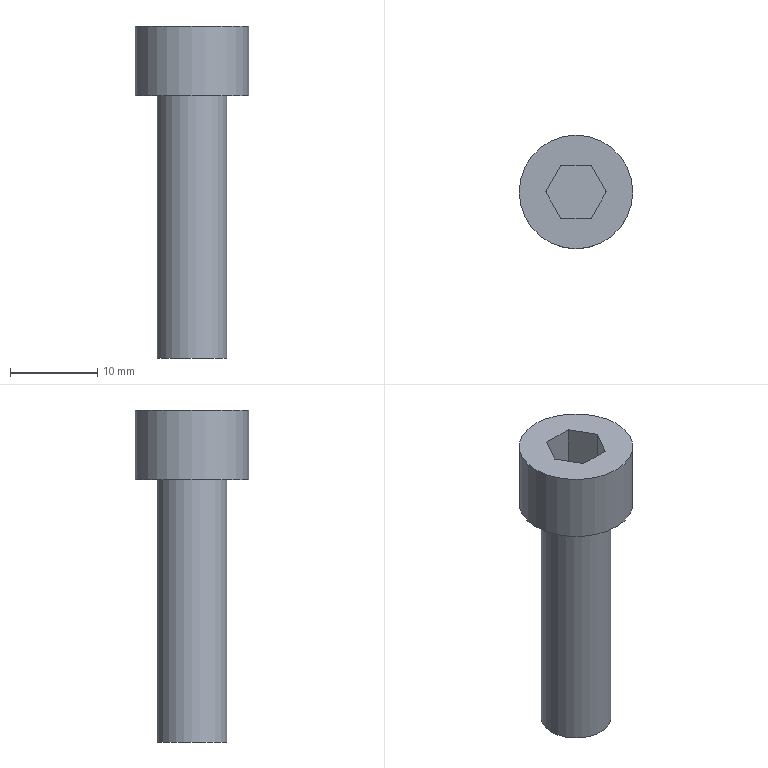Part | STEP file | 冲床-300配套压波_id90_x_t | 1 solid | 12 faces | box 13 x 13 x 38 mm | volume 2405 mm3 | plane 10 | cylinder 2 | commonest cylinder face diameters 8 x1 13 x1
STEP:
#1=CARTESIAN_POINT('',(1171.5,-205.,30.));
#2=VERTEX_POINT('',#1);
#3=CARTESIAN_POINT('',(1165.,-205.,30.));
#4=DIRECTION('',(0.,0.,1.));
#5=DIRECTION('',(1.,0.,0.));
#6=AXIS2_PLACEMENT_3D('',#3,#4,#5);
#7=CIRCLE('',#6,6.5);
#8=EDGE_CURVE('',#2,#2,#7,.T.);
#9=ORIENTED_EDGE('',*,*,#8,.T.);
#10=EDGE_LOOP('',(#9));
#11=FACE_BOUND('',#10,.T.);
#12=CARTESIAN_POINT('',(1166.732,-208.,30.));
#13=VERTEX_POINT('',#12);
#14=CARTESIAN_POINT('',(1163.268,-208.,30.));
#15=VERTEX_POINT('',#14);
#16=CARTESIAN_POINT('',(1163.268,-208.,30.));
#17=DIRECTION('',(-1.,0.,0.));
#18=VECTOR('',#17,1.);
#19=LINE('',#16,#18);
#20=EDGE_CURVE('',#13,#15,#19,.T.);
#21=ORIENTED_EDGE('',*,*,#20,.T.);
#22=CARTESIAN_POINT('',(1161.536,-205.,30.));
#23=VERTEX_POINT('',#22);
#24=CARTESIAN_POINT('',(1161.536,-205.,30.));
#25=DIRECTION('',(-0.5,0.866,0.));
#26=VECTOR('',#25,1.);
#27=LINE('',#24,#26);
#28=EDGE_CURVE('',#15,#23,#27,.T.);
#29=ORIENTED_EDGE('',*,*,#28,.T.);
#30=CARTESIAN_POINT('',(1163.268,-202.,30.));
#31=VERTEX_POINT('',#30);
#32=CARTESIAN_POINT('',(1163.268,-202.,30.));
#33=DIRECTION('',(0.5,0.866,0.));
#34=VECTOR('',#33,1.);
#35=LINE('',#32,#34);
#36=EDGE_CURVE('',#23,#31,#35,.T.);
#37=ORIENTED_EDGE('',*,*,#36,.T.);
#38=CARTESIAN_POINT('',(1166.732,-202.,30.));
#39=VERTEX_POINT('',#38);
#40=CARTESIAN_POINT('',(1166.732,-202.,30.));
#41=DIRECTION('',(1.,0.,0.));
#42=VECTOR('',#41,1.);
#43=LINE('',#40,#42);
#44=EDGE_CURVE('',#31,#39,#43,.T.);
#45=ORIENTED_EDGE('',*,*,#44,.T.);
#46=CARTESIAN_POINT('',(1168.464,-205.,30.));
#47=VERTEX_POINT('',#46);
#48=CARTESIAN_POINT('',(1168.464,-205.,30.));
#49=DIRECTION('',(0.5,-0.866,0.));
#50=VECTOR('',#49,1.);
#51=LINE('',#48,#50);
#52=EDGE_CURVE('',#39,#47,#51,.T.);
#53=ORIENTED_EDGE('',*,*,#52,.T.);
#54=CARTESIAN_POINT('',(1166.732,-208.,30.));
#55=DIRECTION('',(-0.5,-0.866,0.));
#56=VECTOR('',#55,1.);
#57=LINE('',#54,#56);
#58=EDGE_CURVE('',#47,#13,#57,.T.);
#59=ORIENTED_EDGE('',*,*,#58,.T.);
#60=EDGE_LOOP('',(#21,#29,#37,#45,#53,#59));
#61=FACE_BOUND('',#60,.T.);
#62=CARTESIAN_POINT('',(1171.5,-205.,30.));
#63=DIRECTION('',(0.,0.,-1.));
#64=DIRECTION('',(-1.,0.,0.));
#65=AXIS2_PLACEMENT_3D('',#62,#63,#64);
#66=PLANE('',#65);
#67=ADVANCED_FACE('',(#11,#61),#66,.F.);
#68=ORIENTED_EDGE('',*,*,#8,.F.);
#69=EDGE_LOOP('',(#68));
#70=FACE_BOUND('',#69,.T.);
#71=CARTESIAN_POINT('',(1171.5,-205.,22.));
#72=VERTEX_POINT('',#71);
#73=CARTESIAN_POINT('',(1165.,-205.,22.));
#74=DIRECTION('',(0.,0.,1.));
#75=DIRECTION('',(1.,0.,0.));
#76=AXIS2_PLACEMENT_3D('',#73,#74,#75);
#77=CIRCLE('',#76,6.5);
#78=EDGE_CURVE('',#72,#72,#77,.T.);
#79=ORIENTED_EDGE('',*,*,#78,.T.);
#80=EDGE_LOOP('',(#79));
#81=FACE_BOUND('',#80,.T.);
#82=CARTESIAN_POINT('',(1165.,-205.,23.1));
#83=DIRECTION('',(0.,0.,1.));
#84=DIRECTION('',(1.,0.,0.));
#85=AXIS2_PLACEMENT_3D('',#82,#83,#84);
#86=CYLINDRICAL_SURFACE('',#85,6.5);
#87=ADVANCED_FACE('',(#70,#81),#86,.T.);
#88=ORIENTED_EDGE('',*,*,#78,.F.);
#89=EDGE_LOOP('',(#88));
#90=FACE_BOUND('',#89,.T.);
#91=CARTESIAN_POINT('',(1169.,-205.,22.));
#92=VERTEX_POINT('',#91);
#93=CARTESIAN_POINT('',(1165.,-205.,22.));
#94=DIRECTION('',(0.,0.,1.));
#95=DIRECTION('',(1.,0.,0.));
#96=AXIS2_PLACEMENT_3D('',#93,#94,#95);
#97=CIRCLE('',#96,4.);
#98=EDGE_CURVE('',#92,#92,#97,.T.);
#99=ORIENTED_EDGE('',*,*,#98,.T.);
#100=EDGE_LOOP('',(#99));
#101=FACE_BOUND('',#100,.T.);
#102=CARTESIAN_POINT('',(1169.,-205.,22.));
#103=DIRECTION('',(0.,0.,1.));
#104=DIRECTION('',(1.,0.,0.));
#105=AXIS2_PLACEMENT_3D('',#102,#103,#104);
#106=PLANE('',#105);
#107=ADVANCED_FACE('',(#90,#101),#106,.F.);
#108=ORIENTED_EDGE('',*,*,#98,.F.);
#109=EDGE_LOOP('',(#108));
#110=FACE_BOUND('',#109,.T.);
#111=CARTESIAN_POINT('',(1169.,-205.,-8.));
#112=VERTEX_POINT('',#111);
#113=CARTESIAN_POINT('',(1165.,-205.,-8.));
#114=DIRECTION('',(0.,0.,1.));
#115=DIRECTION('',(1.,0.,0.));
#116=AXIS2_PLACEMENT_3D('',#113,#114,#115);
#117=CIRCLE('',#116,4.);
#118=EDGE_CURVE('',#112,#112,#117,.T.);
#119=ORIENTED_EDGE('',*,*,#118,.T.);
#120=EDGE_LOOP('',(#119));
#121=FACE_BOUND('',#120,.T.);
#122=CARTESIAN_POINT('',(1165.,-205.,23.1));
#123=DIRECTION('',(0.,0.,1.));
#124=DIRECTION('',(1.,0.,0.));
#125=AXIS2_PLACEMENT_3D('',#122,#123,#124);
#126=CYLINDRICAL_SURFACE('',#125,4.);
#127=ADVANCED_FACE('',(#110,#121),#126,.T.);
#128=ORIENTED_EDGE('',*,*,#118,.F.);
#129=EDGE_LOOP('',(#128));
#130=FACE_OUTER_BOUND('',#129,.T.);
#131=CARTESIAN_POINT('',(1165.,-205.,-8.));
#132=DIRECTION('',(0.,0.,1.));
#133=DIRECTION('',(1.,0.,0.));
#134=AXIS2_PLACEMENT_3D('',#131,#132,#133);
#135=PLANE('',#134);
#136=ADVANCED_FACE('',(#130),#135,.F.);
#137=ORIENTED_EDGE('',*,*,#20,.F.);
#138=CARTESIAN_POINT('',(1166.732,-208.,24.72));
#139=VERTEX_POINT('',#138);
#140=CARTESIAN_POINT('',(1166.732,-208.,24.72));
#141=DIRECTION('',(0.,0.,1.));
#142=VECTOR('',#141,1.);
#143=LINE('',#140,#142);
#144=EDGE_CURVE('',#139,#13,#143,.T.);
#145=ORIENTED_EDGE('',*,*,#144,.F.);
#146=CARTESIAN_POINT('',(1163.268,-208.,24.72));
#147=VERTEX_POINT('',#146);
#148=CARTESIAN_POINT('',(1163.268,-208.,24.72));
#149=DIRECTION('',(1.,0.,0.));
#150=VECTOR('',#149,1.);
#151=LINE('',#148,#150);
#152=EDGE_CURVE('',#147,#139,#151,.T.);
#153=ORIENTED_EDGE('',*,*,#152,.F.);
#154=CARTESIAN_POINT('',(1163.268,-208.,24.72));
#155=DIRECTION('',(0.,0.,1.));
#156=VECTOR('',#155,1.);
#157=LINE('',#154,#156);
#158=EDGE_CURVE('',#147,#15,#157,.T.);
#159=ORIENTED_EDGE('',*,*,#158,.T.);
#160=EDGE_LOOP('',(#137,#145,#153,#159));
#161=FACE_OUTER_BOUND('',#160,.T.);
#162=CARTESIAN_POINT('',(1163.268,-208.,24.72));
#163=DIRECTION('',(0.,1.,0.));
#164=DIRECTION('',(1.,0.,0.));
#165=AXIS2_PLACEMENT_3D('',#162,#163,#164);
#166=PLANE('',#165);
#167=ADVANCED_FACE('',(#161),#166,.T.);
#168=ORIENTED_EDGE('',*,*,#58,.F.);
#169=CARTESIAN_POINT('',(1168.464,-205.,24.72));
#170=VERTEX_POINT('',#169);
#171=CARTESIAN_POINT('',(1168.464,-205.,24.72));
#172=DIRECTION('',(0.,0.,1.));
#173=VECTOR('',#172,1.);
#174=LINE('',#171,#173);
#175=EDGE_CURVE('',#170,#47,#174,.T.);
#176=ORIENTED_EDGE('',*,*,#175,.F.);
#177=CARTESIAN_POINT('',(1166.732,-208.,24.72));
#178=DIRECTION('',(0.5,0.866,0.));
#179=VECTOR('',#178,1.);
#180=LINE('',#177,#179);
#181=EDGE_CURVE('',#139,#170,#180,.T.);
#182=ORIENTED_EDGE('',*,*,#181,.F.);
#183=ORIENTED_EDGE('',*,*,#144,.T.);
#184=EDGE_LOOP('',(#168,#176,#182,#183));
#185=FACE_OUTER_BOUND('',#184,.T.);
#186=CARTESIAN_POINT('',(1166.732,-208.,24.72));
#187=DIRECTION('',(-0.866,0.5,0.));
#188=DIRECTION('',(0.5,0.866,0.));
#189=AXIS2_PLACEMENT_3D('',#186,#187,#188);
#190=PLANE('',#189);
#191=ADVANCED_FACE('',(#185),#190,.T.);
#192=ORIENTED_EDGE('',*,*,#52,.F.);
#193=CARTESIAN_POINT('',(1166.732,-202.,24.72));
#194=VERTEX_POINT('',#193);
#195=CARTESIAN_POINT('',(1166.732,-202.,24.72));
#196=DIRECTION('',(0.,0.,1.));
#197=VECTOR('',#196,1.);
#198=LINE('',#195,#197);
#199=EDGE_CURVE('',#194,#39,#198,.T.);
#200=ORIENTED_EDGE('',*,*,#199,.F.);
#201=CARTESIAN_POINT('',(1168.464,-205.,24.72));
#202=DIRECTION('',(-0.5,0.866,0.));
#203=VECTOR('',#202,1.);
#204=LINE('',#201,#203);
#205=EDGE_CURVE('',#170,#194,#204,.T.);
#206=ORIENTED_EDGE('',*,*,#205,.F.);
#207=ORIENTED_EDGE('',*,*,#175,.T.);
#208=EDGE_LOOP('',(#192,#200,#206,#207));
#209=FACE_OUTER_BOUND('',#208,.T.);
#210=CARTESIAN_POINT('',(1168.464,-205.,24.72));
#211=DIRECTION('',(-0.866,-0.5,0.));
#212=DIRECTION('',(-0.5,0.866,0.));
#213=AXIS2_PLACEMENT_3D('',#210,#211,#212);
#214=PLANE('',#213);
#215=ADVANCED_FACE('',(#209),#214,.T.);
#216=ORIENTED_EDGE('',*,*,#44,.F.);
#217=CARTESIAN_POINT('',(1163.268,-202.,24.72));
#218=VERTEX_POINT('',#217);
#219=CARTESIAN_POINT('',(1163.268,-202.,24.72));
#220=DIRECTION('',(0.,0.,1.));
#221=VECTOR('',#220,1.);
#222=LINE('',#219,#221);
#223=EDGE_CURVE('',#218,#31,#222,.T.);
#224=ORIENTED_EDGE('',*,*,#223,.F.);
#225=CARTESIAN_POINT('',(1166.732,-202.,24.72));
#226=DIRECTION('',(-1.,0.,0.));
#227=VECTOR('',#226,1.);
#228=LINE('',#225,#227);
#229=EDGE_CURVE('',#194,#218,#228,.T.);
#230=ORIENTED_EDGE('',*,*,#229,.F.);
#231=ORIENTED_EDGE('',*,*,#199,.T.);
#232=EDGE_LOOP('',(#216,#224,#230,#231));
#233=FACE_OUTER_BOUND('',#232,.T.);
#234=CARTESIAN_POINT('',(1166.732,-202.,24.72));
#235=DIRECTION('',(0.,-1.,0.));
#236=DIRECTION('',(-1.,0.,0.));
#237=AXIS2_PLACEMENT_3D('',#234,#235,#236);
#238=PLANE('',#237);
#239=ADVANCED_FACE('',(#233),#238,.T.);
#240=ORIENTED_EDGE('',*,*,#36,.F.);
#241=CARTESIAN_POINT('',(1161.536,-205.,24.72));
#242=VERTEX_POINT('',#241);
#243=CARTESIAN_POINT('',(1161.536,-205.,24.72));
#244=DIRECTION('',(0.,0.,1.));
#245=VECTOR('',#244,1.);
#246=LINE('',#243,#245);
#247=EDGE_CURVE('',#242,#23,#246,.T.);
#248=ORIENTED_EDGE('',*,*,#247,.F.);
#249=CARTESIAN_POINT('',(1163.268,-202.,24.72));
#250=DIRECTION('',(-0.5,-0.866,0.));
#251=VECTOR('',#250,1.);
#252=LINE('',#249,#251);
#253=EDGE_CURVE('',#218,#242,#252,.T.);
#254=ORIENTED_EDGE('',*,*,#253,.F.);
#255=ORIENTED_EDGE('',*,*,#223,.T.);
#256=EDGE_LOOP('',(#240,#248,#254,#255));
#257=FACE_OUTER_BOUND('',#256,.T.);
#258=CARTESIAN_POINT('',(1163.268,-202.,24.72));
#259=DIRECTION('',(0.866,-0.5,0.));
#260=DIRECTION('',(-0.5,-0.866,0.));
#261=AXIS2_PLACEMENT_3D('',#258,#259,#260);
#262=PLANE('',#261);
#263=ADVANCED_FACE('',(#257),#262,.T.);
#264=ORIENTED_EDGE('',*,*,#28,.F.);
#265=ORIENTED_EDGE('',*,*,#158,.F.);
#266=CARTESIAN_POINT('',(1161.536,-205.,24.72));
#267=DIRECTION('',(0.5,-0.866,0.));
#268=VECTOR('',#267,1.);
#269=LINE('',#266,#268);
#270=EDGE_CURVE('',#242,#147,#269,.T.);
#271=ORIENTED_EDGE('',*,*,#270,.F.);
#272=ORIENTED_EDGE('',*,*,#247,.T.);
#273=EDGE_LOOP('',(#264,#265,#271,#272));
#274=FACE_OUTER_BOUND('',#273,.T.);
#275=CARTESIAN_POINT('',(1161.536,-205.,24.72));
#276=DIRECTION('',(0.866,0.5,0.));
#277=DIRECTION('',(0.5,-0.866,0.));
#278=AXIS2_PLACEMENT_3D('',#275,#276,#277);
#279=PLANE('',#278);
#280=ADVANCED_FACE('',(#274),#279,.T.);
#281=ORIENTED_EDGE('',*,*,#152,.T.);
#282=ORIENTED_EDGE('',*,*,#181,.T.);
#283=ORIENTED_EDGE('',*,*,#205,.T.);
#284=ORIENTED_EDGE('',*,*,#229,.T.);
#285=ORIENTED_EDGE('',*,*,#253,.T.);
#286=ORIENTED_EDGE('',*,*,#270,.T.);
#287=EDGE_LOOP('',(#281,#282,#283,#284,#285,#286));
#288=FACE_OUTER_BOUND('',#287,.T.);
#289=CARTESIAN_POINT('',(1165.,-205.,24.72));
#290=DIRECTION('',(0.,0.,-1.));
#291=DIRECTION('',(-1.,0.,0.));
#292=AXIS2_PLACEMENT_3D('',#289,#290,#291);
#293=PLANE('',#292);
#294=ADVANCED_FACE('',(#288),#293,.F.);
#295=CLOSED_SHELL('',(#67,#87,#107,#127,#136,#167,#191,#215,#239,#263,#280,#294));
#296=MANIFOLD_SOLID_BREP('',#295);
#297=(LENGTH_UNIT()NAMED_UNIT(*)SI_UNIT(.MILLI.,.METRE.));
#298=UNCERTAINTY_MEASURE_WITH_UNIT(LENGTH_MEASURE(0.00002),#297,'','');
#299=(NAMED_UNIT(*)PLANE_ANGLE_UNIT()SI_UNIT($,.RADIAN.));
#300=PLANE_ANGLE_MEASURE_WITH_UNIT(PLANE_ANGLE_MEASURE(0.01745),#299);
#301=DIMENSIONAL_EXPONENTS(0.,0.,0.,0.,0.,0.,0.);
#302=(CONVERSION_BASED_UNIT('DEGREE',#300)NAMED_UNIT(#301)PLANE_ANGLE_UNIT());
#303=(NAMED_UNIT(*)SI_UNIT($,.STERADIAN.)SOLID_ANGLE_UNIT());
#304=(GEOMETRIC_REPRESENTATION_CONTEXT(3)GLOBAL_UNCERTAINTY_ASSIGNED_CONTEXT((#298))GLOBAL_UNIT_ASSIGNED_CONTEXT((#297,#302,#303))REPRESENTATION_CONTEXT('',''));
#305=ADVANCED_BREP_SHAPE_REPRESENTATION('',(#296),#304);